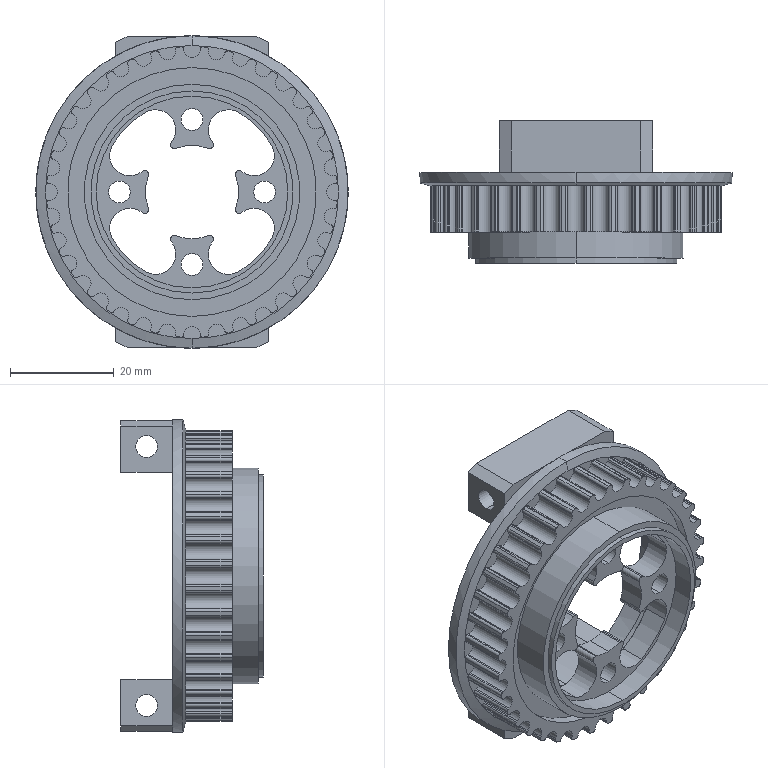Part | SolidWorks | features ICE 4, Chamfer 2, CirPattern 1, HoleWzd 1, Revolution 1 | 1 solid | 356 faces | box 60.296 x 27.5 x 60.296 mm | volume 17224 mm3 | cylinder 248 | plane 106 | cone 2 | commonest cylinder face diameters 0.96 x90 3.12 x53 56.16 x36 1.44 x12 4.2 x12 7.8 x12